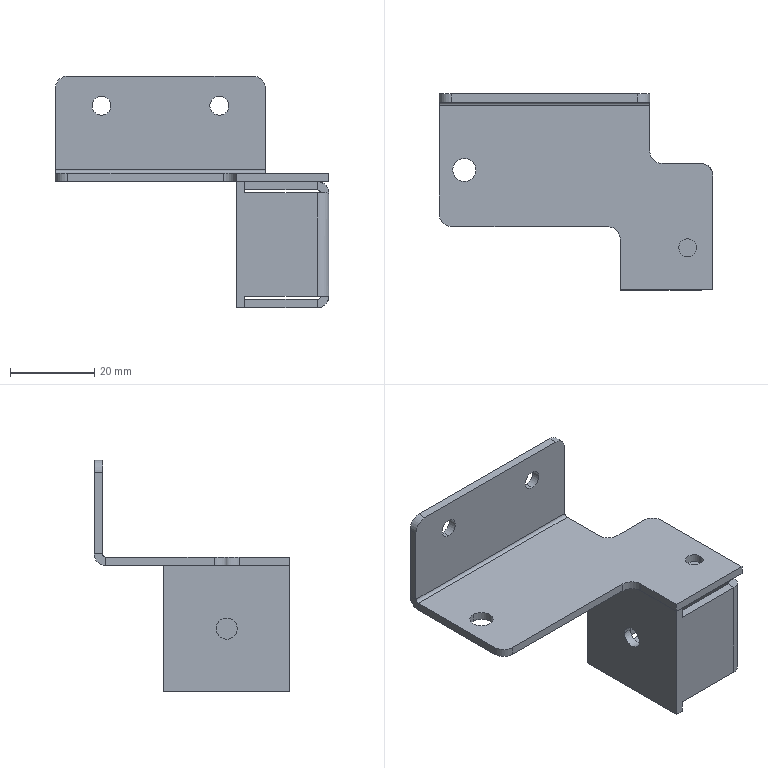Part | SolidWorks | features HoleWzd 4, ICE 3, EdgeFlange 2, FlatPattern 2, SMBaseFlange 2, SheetMetal 2, Cut 1, Fillet 1 | 2 solids | 70 faces | box 65 x 46.5 x 55 mm | volume 13185 mm3 | plane 34 | cylinder 28 | spline 8 | commonest cylinder face diameters 5.5 x9 6 x6 1.5 x5 4.5 x4 4.2 x2 5 x2